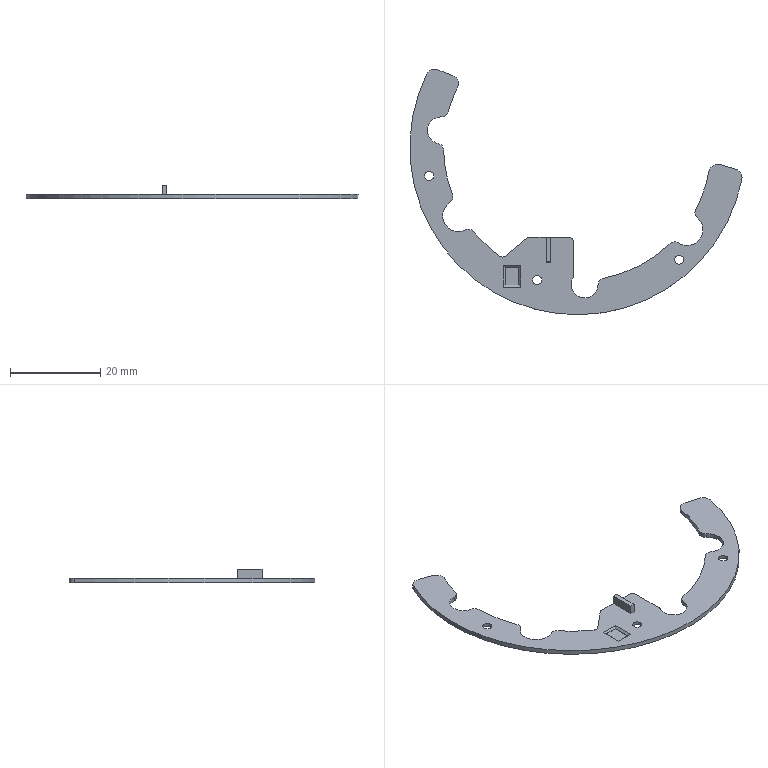Part | STEP file | TQ-DD-1105-THCover1010_デフォルト | 1 solid | 64 faces | box 73.74 x 54.492 x 3 mm | volume 881.003 mm3 | cylinder 41 | plane 23 | commonest cylinder face diameters 2 x9 3 x9 5 x6 59.4 x5 4 x4 6 x4